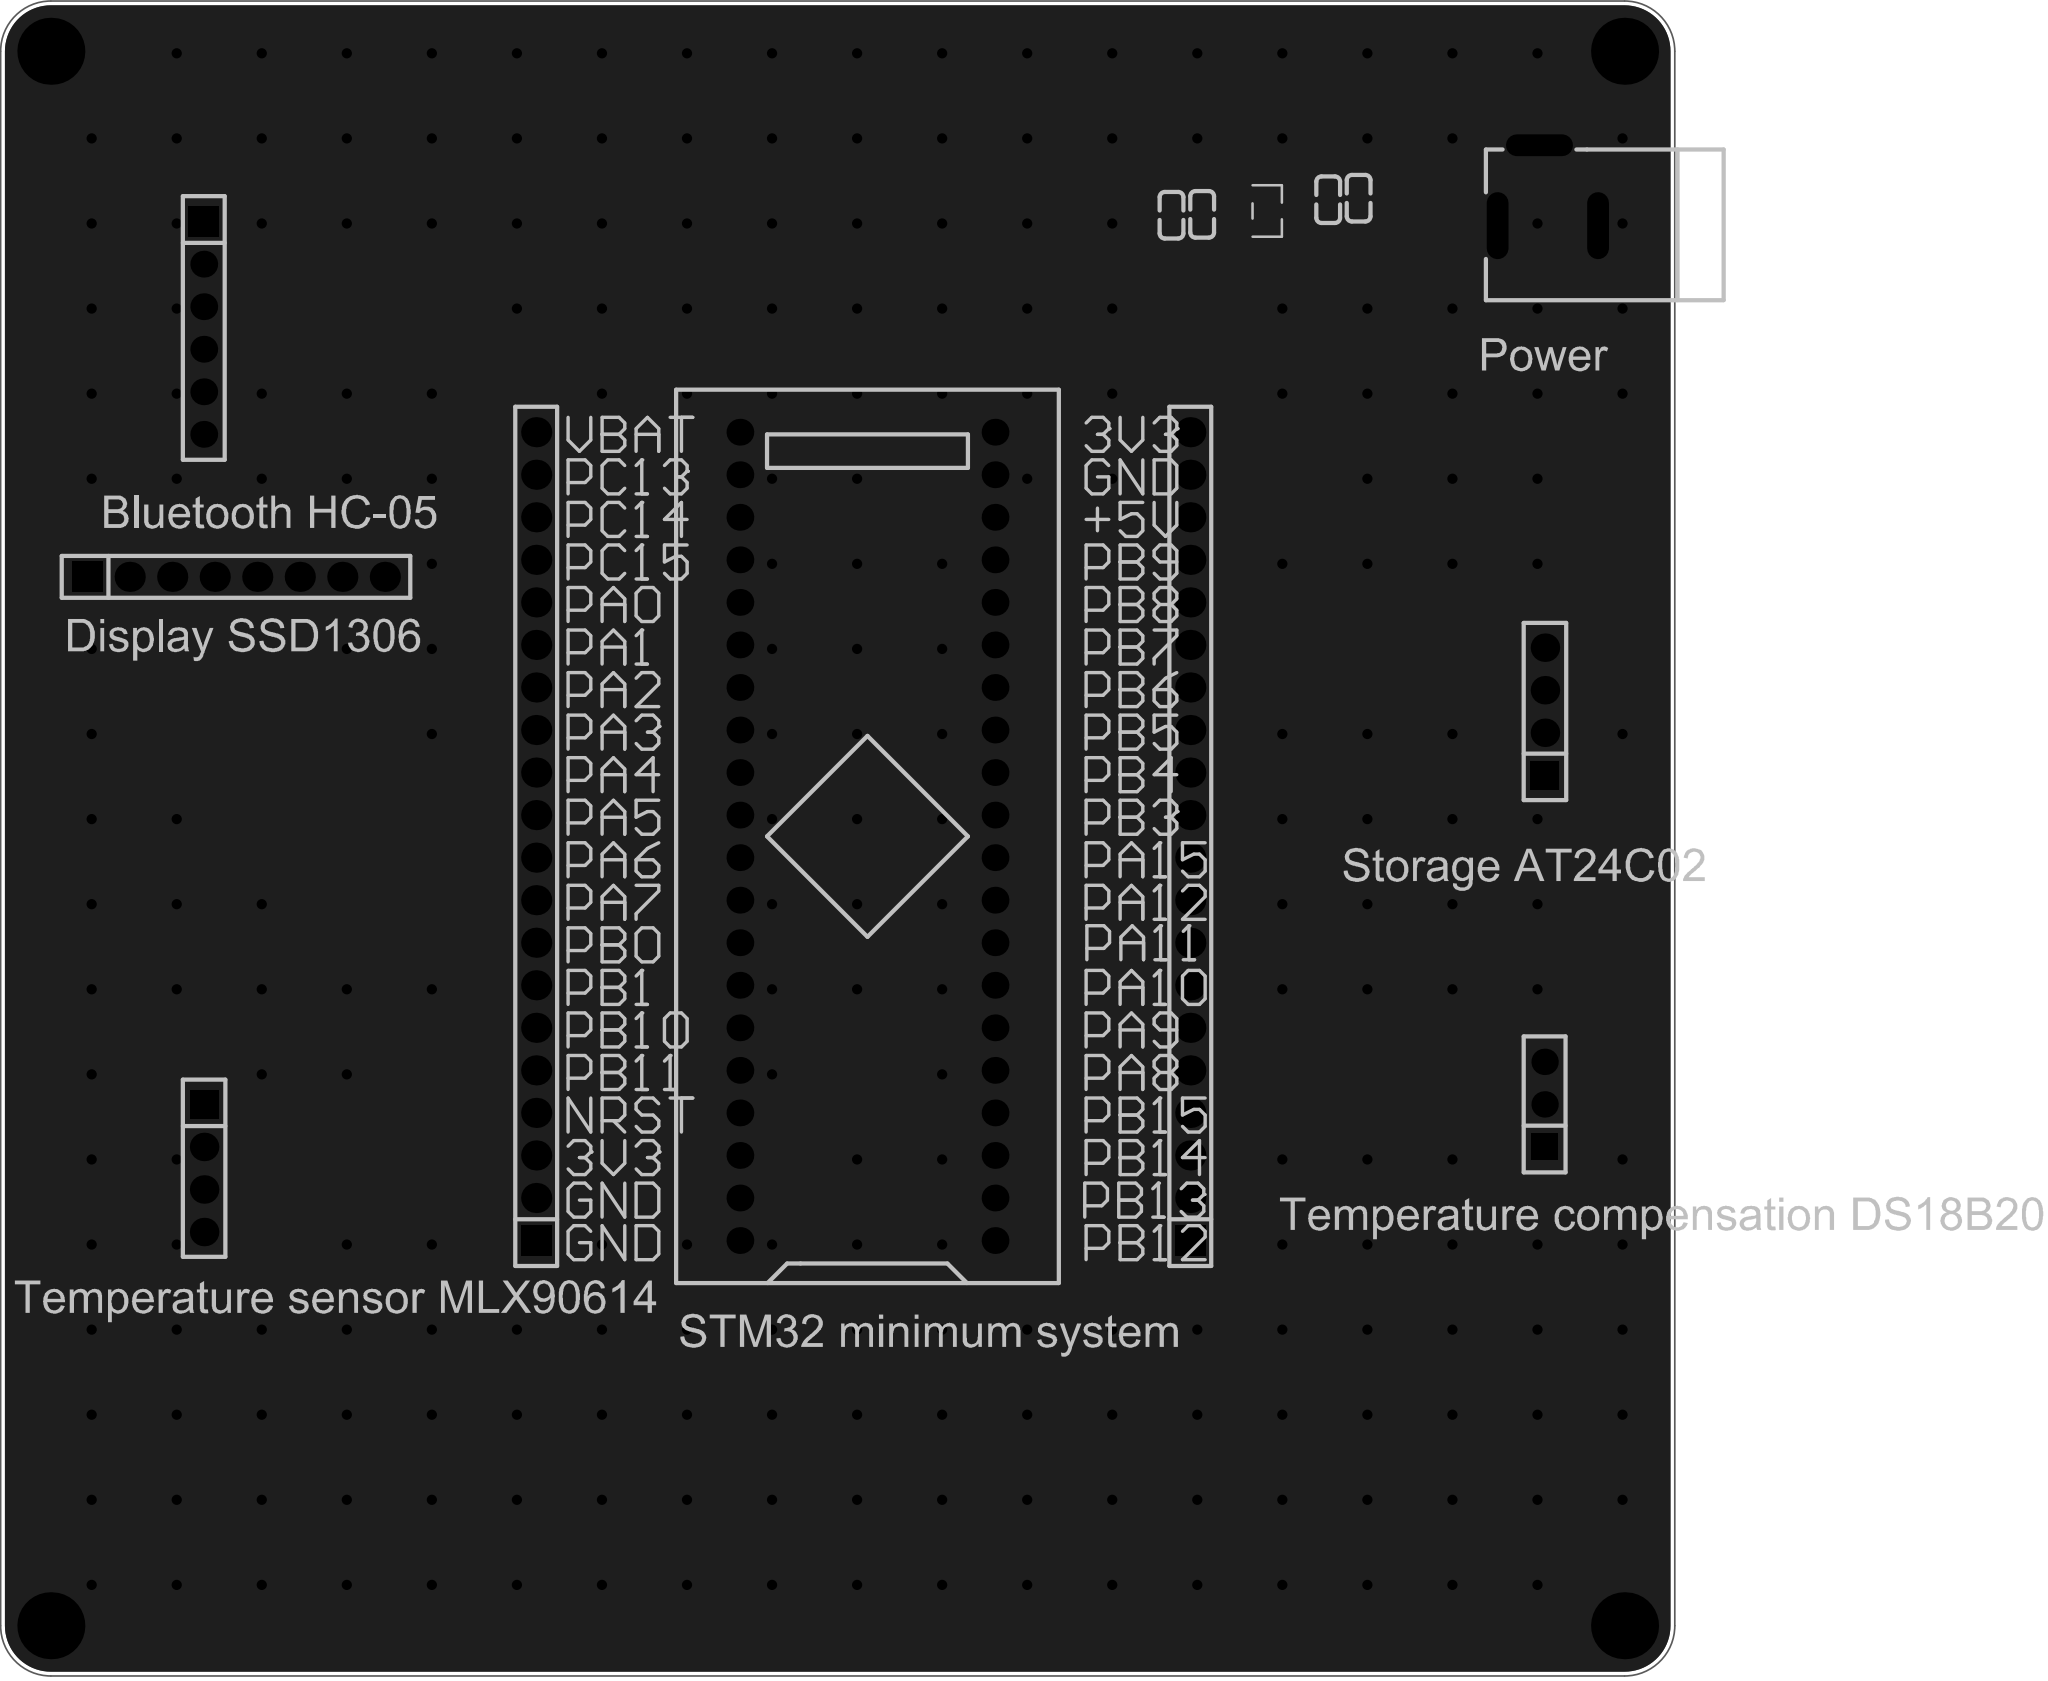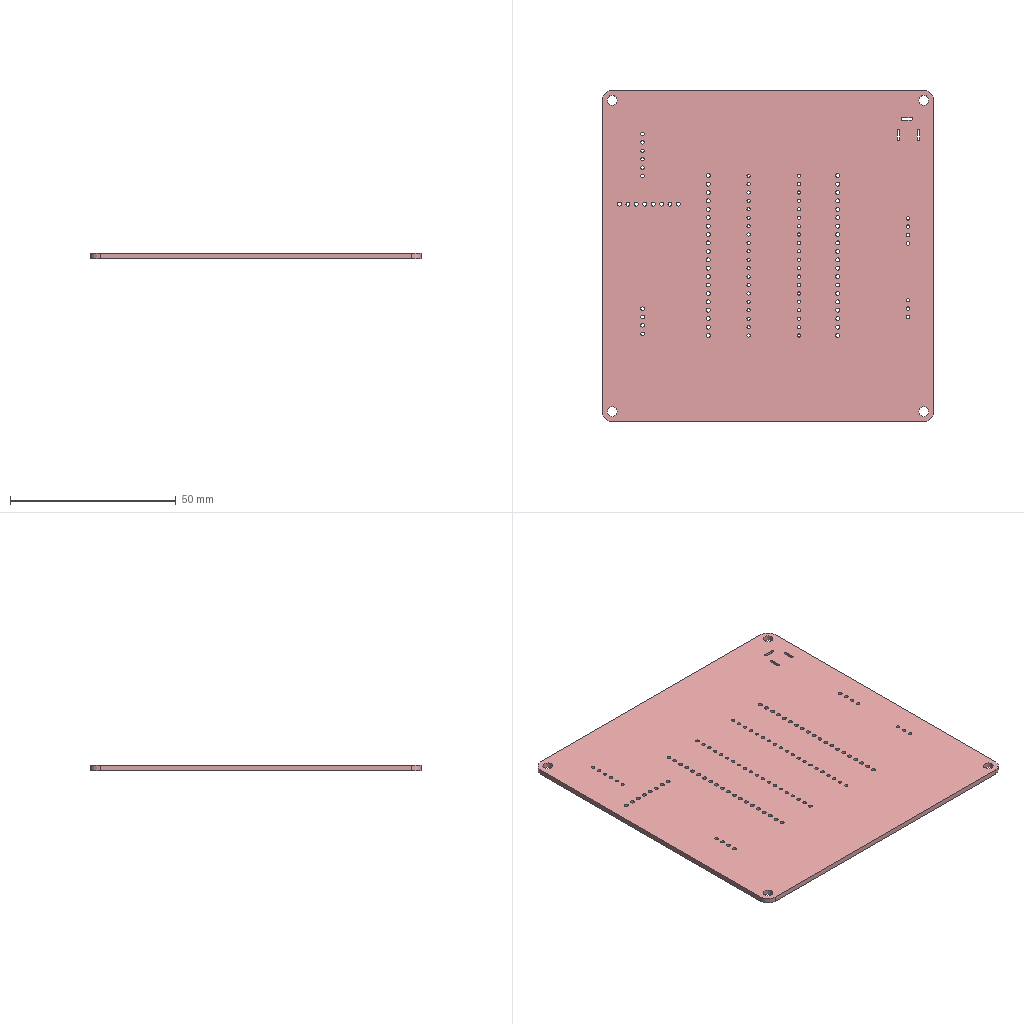Circuit board layout | Altium Designer | box 100 x 100 x 1.6 mm
Layer stack:
# Altium Designer layer stack of  (unit mm; dielectric type: 0 none, 1 core, 2 prepreg, 3 surface material)
index,name,kind,layer,copper_thickness_mm,dielectric_type,dielectric_thickness_mm,dielectric_material,dielectric_constant
0,Top Paste Mask Layer,other,,,,,,
1,Top Silkscreen Layer,other,,,,,,
2,Top Solder Mask Layer,dielectric,,,3,0.01,,3.3
3,Top Layer,copper,Top Layer,0.035,,,,
4,Dielectric1,dielectric,,,3,1.51,FR4,4.5
5,Bottom Layer,copper,Bottom Layer,0.035,,,,
6,Bottom Solder Mask Layer,dielectric,,,3,0.01,,3.3
7,Bottom Silkscreen Layer,other,,,,,,
8,Bottom Paste Mask Layer,other,,,,,,
# drill layer pairs: low layer,high layer
drill_pair,Top Layer,Bottom Layer
Part placement:
Designator,Comment,Layer,Footprint,Center-X(mm),Center-Y(mm),Rotation
U1,STM32F103C8T6-Card,TopLayer,CONN-TH_L53.3-W22.9_STM32F103C8T6-CARD,132.334,129.032,90
H1,,TopLayer,HDR-TH_20P-P2.54-V-F,151.617,129.032,90
H2,,TopLayer,HDR-TH_20P-P2.54-V-F,112.546,129.032,90
C1,10uF,TopLayer,C0603,161.671,167.132,270
C2,100nF,TopLayer,C0603,159.854,167.043,270
C3,10uF,TopLayer,C0603,152.326,166.169,270
C4,100nF,TopLayer,C0603,150.495,166.116,270
DC1,,TopLayer,DC-2.0,172.974,167.894,0
H3,,TopLayer,HDR-TH_4P-P2.54-V-F,92.71,109.22,270
H4,,TopLayer,HDR-TH_6P-P2.54-V-F,92.69,159.385,270
H5,,TopLayer,HDR-TH_8P-P2.54-V-F-1,94.615,144.526,0
H6,,TopLayer,HDR-TH_4P-P2.54-V-F,172.8,136.487,90
H7,,TopLayer,HDR-TH_3P-P2.54-V-F,172.78,113.03,90
U2,HT7333,TopLayer,SOT-23-3_L2.9-W1.6-P1.90-LS2.8-BR,156.21,166.37,180
Pad and via stacks:
# Altium Designer via and pad stacks of  (unit mm). Each distinct definition once, with the count of objects using it.
# via: kind,start_layer,end_layer,hole_mm,diameter_mm,mode(0 simple;1 top-mid-bottom;2 full stack),diameter_per_layer,count,example_net
# pad: kind,layer,hole_mm,hole_type(0 round;1 square;2 slot),plating,top_size,top_shape(1 round;2 rect;3 octagon;9 rounded rect),mid_size,bottom_size,mode,footprint,size_per_layer,count,example
pad,Multi-Layer,3,0,plated,4x4,1,4x4,4x4,0,,,4,1
pad,Multi-Layer,1,0,plated,1.6x1.6,1,1.6x1.6,1.6x1.6,0,CONN-TH_L53.3-W22.9_STM32F103C8T6-CARD,,40,U1.1
pad,Multi-Layer,1.2,0,plated,1.8x1.8,2,1.8x1.8,1.8x1.8,0,HDR-TH_20P-P2.54-V-F,,2,H1.1
pad,Multi-Layer,1.2,0,plated,1.8x1.8,1,1.8x1.8,1.8x1.8,0,HDR-TH_20P-P2.54-V-F,,38,H1.2
pad,Multi-Layer,0.8001,2,plated,4x1.3,1,4x1.3,4x1.3,0,DC-2.0,,3,DC1.2
pad,Multi-Layer,1.1,0,plated,1.7x1.7,2,1.7x1.7,1.7x1.7,0,HDR-TH_4P-P2.54-V-F,,2,H3.1
pad,Multi-Layer,1.1,0,plated,1.7x1.7,1,1.7x1.7,1.7x1.7,0,HDR-TH_4P-P2.54-V-F,,6,H3.2
pad,Multi-Layer,1.02,0,plated,1.6x1.6,1,1.6x1.6,1.6x1.6,0,HDR-TH_6P-P2.54-V-F,,5,H4.6
pad,Multi-Layer,1.02,0,plated,1.8x1.8,2,1.8x1.8,1.8x1.8,0,HDR-TH_6P-P2.54-V-F,,1,H4.1
pad,Multi-Layer,1.2,0,plated,1.8x1.8,2,1.8x1.8,1.8x1.8,0,HDR-TH_8P-P2.54-V-F-1,,1,H5.1
pad,Multi-Layer,1.2,0,plated,1.8x1.8,1,1.8x1.8,1.8x1.8,0,HDR-TH_8P-P2.54-V-F-1,,7,H5.2
pad,Multi-Layer,1.02,0,plated,1.575x1.575,1,1.575x1.575,1.575x1.575,0,HDR-TH_3P-P2.54-V-F,,2,H7.3
pad,Multi-Layer,1.02,0,plated,1.575x1.575,2,1.575x1.575,1.575x1.575,0,HDR-TH_3P-P2.54-V-F,,1,H7.1
pad,Top Layer,0,0,plated,0.8x0.9,2,0.8x0.9,0.8x0.9,0,C0603,,8,C1.2
pad,Top Layer,0,0,plated,1.07x0.6,2,1.07x0.6,1.07x0.6,0,SOT-23-3_L2.9-W1.6-P1.90-LS2.8-BR,,3,U2.1
via,Top Layer,Bottom Layer,0.3048,0.61,0,,250,GND
Copper pours:
name,layer,net,type(0 solid;1 hatched;2 none)
Bottom Layer-GND,Bottom Layer,GND,0
Top Layer-GND,Top Layer,GND,0